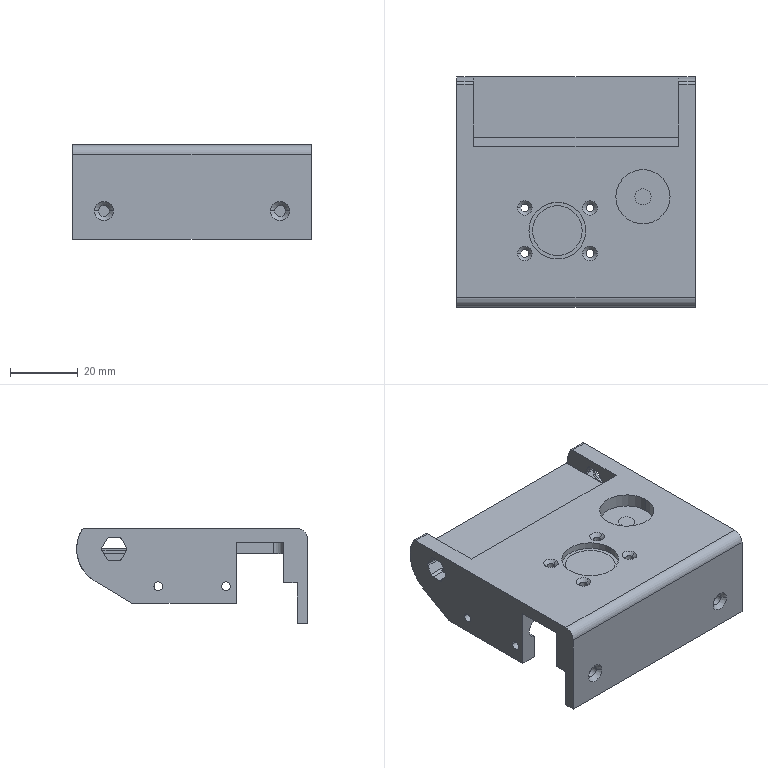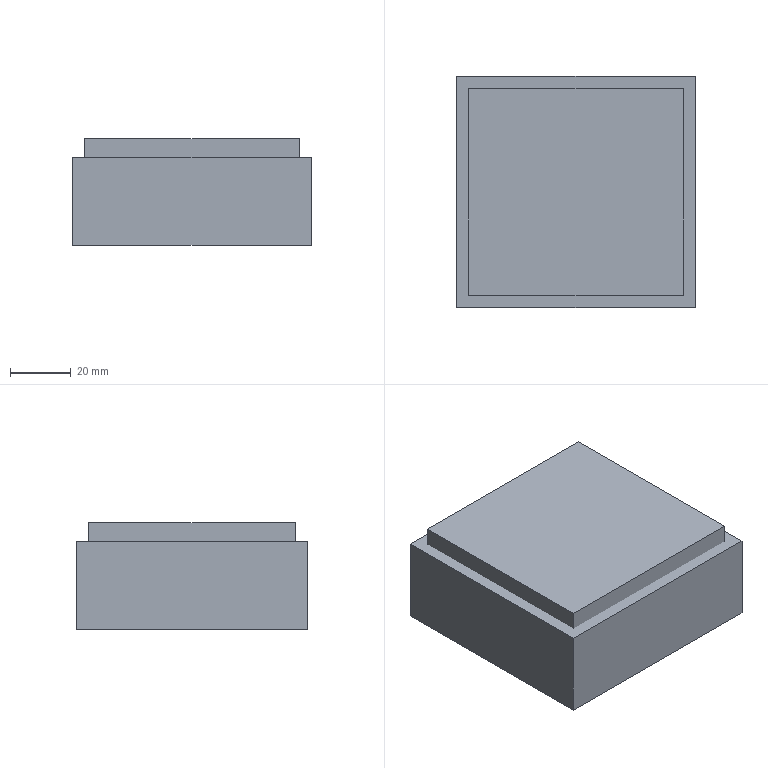CAM job | NX | 3+2 milling, drilling | part box 70.5 x 68.1 x 28 mm | stock box 78.5 x 76.1 x 35 mm
Tools:
number,name,description,diameter,corner_radius,flute_length,length,flutes
1,D63,Milling Tool-5 Parameters,63.0,0.0,50.0,75.0,2
7,D6A45,Milling Tool-5 Parameters,6.0,0.0,3.0,3.0,2
13,3.2ZT,Drilling Tool,3.2,0.0,35.0,50.0,2
12,2.3ZT,Drilling Tool,2.3,0.0,35.0,50.0,2
14,4.8ZT,Drilling Tool,4.8,0.0,35.0,50.0,2
10,D10,Milling Tool-5 Parameters,10.0,0.0,50.0,75.0,2
11,D10JING,Milling Tool-5 Parameters,10.0,0.0,50.0,75.0,2
9,D2R0.5,Milling Tool-5 Parameters,2.0,0.5,50.0,75.0,2
4,D4,Milling Tool-5 Parameters,4.0,0.0,50.0,75.0,2
6,D6,Milling Tool-5 Parameters,6.0,0.0,50.0,75.0,2
2,D2,Milling Tool-5 Parameters,2.0,0.0,50.0,75.0,2
5,D6R0.5,Milling Tool-5 Parameters,6.0,0.5,50.0,75.0,2
16,6.0ZT,Drilling Tool,6.0,0.0,35.0,50.0,2
12,2.6ZT,Drilling Tool,2.6,0.0,35.0,50.0,2
17,2.5ZT,Drilling Tool,2.5,0.0,35.0,50.0,2
Operations:
program,operation,operation_type,tool,method,geometry_group,spindle_rpm,surface_speed,feed_per_tooth,feed_cut,feed_plunge,cut_length_mm,path_length_mm,cut_time_min,machine_time_min
1-75-75-25毛胚,FLOOR_WALL,VolumeBased25DMillingOperation,D63,METHOD,A,6500.0,1286.0,0.0962,1250.0,100.0,482.597,536.597,0.3861,0.3915
1-75-75-25毛胚,DRILLING,Operation,D6A45,METHOD,A,3500.0,43.0,0.0357,250.0,0.0,30.9,223.35,0.1236,0.1428
1-75-75-25毛胚,DRILLING_COPY_COPY,Operation,2.3ZT,METHOD,A,2500.0,19.0,0.024,120.0,0.0,36.764,189.628,0.3064,0.3217
1-75-75-25毛胚,DRILLING_COPY_COPY_COPY,Operation,4.8ZT,METHOD,A,2500.0,19.0,0.024,120.0,0.0,13.442,86.884,0.112,0.1194
1-75-75-25毛胚,ADAPTIVE_MILLING,CavityMilling,D10,METHOD,A,9500.0,298.0,0.1579,3000.0,1000.0,5837.721,7450.176,1.978,2.139
1-75-75-25毛胚,HOLE_MILLING,CylinderMilling,D10,METHOD,A,9500.0,298.0,0.1053,2000.0,100.0,225.87,378.029,0.1129,0.1282
1-75-75-25毛胚,HOLE_MILLING_COPY,CylinderMilling,D10,METHOD,A,9500.0,298.0,0.1053,2000.0,100.0,65.455,130.955,0.0327,0.0393
1-75-75-25毛胚,ZLEVEL_PROFILE_1,ZLevelMilling,D10JING,METHOD,A,9500.0,298.0,0.0526,1000.0,100.0,635.228,748.794,0.6352,0.6466
1-75-75-25毛胚,ZLEVEL_PROFILE_1_COPY,ZLevelMilling,D10JING,METHOD,A,9500.0,298.0,0.0526,1000.0,100.0,30.207,95.207,0.0302,0.0367
1-75-75-25毛胚,ZLEVEL_PROFILE_1_COPY_COPY,ZLevelMilling,D10JING,METHOD,A,9500.0,298.0,0.0526,1000.0,100.0,32.414,93.414,0.0324,0.0385
1-75-75-25毛胚,ZLEVEL_PROFILE_1_COPY_COPY_COPY,ZLevelMilling,D10JING,METHOD,A,9500.0,298.0,0.0526,1000.0,100.0,25.226,87.226,0.0252,0.0314
1-75-75-25毛胚,FLOOR_WALL_1,VolumeBased25DMillingOperation,D10JING,METHOD,A,9500.0,298.0,0.0658,1250.0,100.0,323.3,477.906,0.2586,0.2741
1-75-75-25毛胚,CAVITY_MILL_COPY_COPY,CavityMilling,D4,METHOD,A,9500.0,119.0,0.0737,1400.0,1000.0,345.486,803.476,0.2655,0.3113
1-75-75-25毛胚,CAVITY_MILL_COPY_COPY_COPY,CavityMilling,D2,METHOD,A,9500.0,59.0,0.0526,1000.0,1000.0,429.881,1061.337,0.4299,0.493
1-75-75-25毛胚,ZLEVEL_PROFILE_COPY_COPY_1_1_COPY_1,ZLevelMilling,D2R0.5,METHOD,A,9500.0,59.0,0.1053,2000.0,1000.0,4164.504,4229.096,2.083,2.09
1-75-75-25毛胚,ZLEVEL_PROFILE_COPY_COPY_1_COPY_1,ZLevelMilling,D6R0.5,METHOD,A,9500.0,179.0,0.1579,3000.0,1000.0,4405.43,4466.937,1.47,1.476
1-75-75-25毛胚,ZLEVEL_PROFILE_COPY_COPY_1_COPY_1_COPY,ZLevelMilling,D6R0.5,METHOD,A,9500.0,179.0,0.1579,3000.0,1000.0,1807.575,1989.442,0.6058,0.624
1-75-75-25毛胚,ZLEVEL_PROFILE_1_COPY_1_COPY_COPY_COPY_1,ZLevelMilling,D6A45,METHOD,A,9500.0,179.0,0.0526,1000.0,100.0,274.576,779.626,0.2746,0.3251
1-75-75-25毛胚,ZLEVEL_PROFILE_1_COPY_1_COPY_COPY_COPY_1_COPY,ZLevelMilling,D6A45,METHOD,A,9500.0,179.0,0.0526,1000.0,100.0,14.339,82.339,0.0143,0.0211
2,DRILLING_COPY,Operation,D6A45,METHOD,B,3500.0,43.0,0.0357,250.0,0.0,10.3,142.676,0.0412,0.0544
2,DRILLING_COPY_COPY_COPY_COPY,Operation,6.0ZT,METHOD,B,2500.0,19.0,0.024,120.0,0.0,82.705,287.486,0.6892,0.7097
3,DRILLING_1,Operation,D6A45,METHOD,C,3500.0,43.0,0.0357,250.0,0.0,11.6,138.286,0.0464,0.0591
3,DRILLING_COPY_COPY_1,Operation,3.2ZT,METHOD,C,2500.0,19.0,0.024,120.0,0.0,16.923,148.932,0.141,0.1542
4,DRILLING_COPY_1,Operation,D6A45,METHOD,D,3500.0,43.0,0.0357,250.0,0.0,8.8,100.824,0.0352,0.0444
4,DRILLING_COPY_COPY_COPY_1,Operation,2.6ZT,METHOD,D,2500.0,19.0,0.024,120.0,0.0,20.562,124.348,0.1714,0.1817
4,ZLEVEL_PROFILE_COPY,ZLevelMilling,D2,METHOD,D,9500.0,59.0,0.0526,1000.0,1000.0,595.828,658.828,0.5958,0.6021
4,ZLEVEL_PROFILE_1_COPY_1_COPY_COPY_COPY_1_COPY_COPY,ZLevelMilling,D6A45,METHOD,D,9500.0,179.0,0.0526,1000.0,100.0,33.118,264.656,0.0331,0.0563
5,DRILLING_COPY_2,Operation,D6A45,METHOD,E,3500.0,43.0,0.0357,250.0,0.0,12.0,156.733,0.048,0.0625
5,DRILLING_COPY_COPY_COPY_2,Operation,2.5ZT,METHOD,E,2500.0,19.0,0.024,120.0,0.0,11.5,83.0,0.0958,0.103
5,DRILLING_COPY_COPY_COPY_1_COPY,Operation,2.6ZT,METHOD,E,2500.0,19.0,0.024,120.0,0.0,10.281,80.562,0.0857,0.0927
5,ZLEVEL_PROFILE_COPY_COPY,ZLevelMilling,D4,METHOD,E,9500.0,119.0,0.0684,1300.0,1000.0,252.739,316.306,0.2058,0.2122
5,ZLEVEL_PROFILE_COPY_COPY_1,ZLevelMilling,D2R0.5,METHOD,E,9500.0,59.0,0.0789,1500.0,1000.0,1038.406,1101.906,0.6993,0.7056
5,ZLEVEL_PROFILE_1_COPY_1_COPY_COPY_COPY_1_COPY_COPY_COPY,ZLevelMilling,D6A45,METHOD,E,9500.0,179.0,0.0526,1000.0,100.0,36.649,315.718,0.0366,0.0646
5,刀补4,ZLevelMilling,D4,METHOD,E,9500.0,119.0,0.0526,1000.0,100.0,17.875,76.34,0.0179,0.0237
6,FLOOR_WALL_COPY,VolumeBased25DMillingOperation,D63,METHOD,F,6500.0,1286.0,0.0962,1250.0,100.0,2236.479,2844.263,1.789,1.85
6,FLOOR_WALL_2,VolumeBased25DMillingOperation,D10,METHOD,F,9500.0,298.0,0.1579,3000.0,1000.0,5409.407,5475.107,1.807,1.814
6,ADAPTIVE_MILLING_COPY,CavityMilling,D10,METHOD,F,9500.0,298.0,0.1579,3000.0,1000.0,10554.564,17811.647,3.646,4.372
6,HOLE_MILLING_COPY_COPY,CylinderMilling,D10,METHOD,F,9500.0,298.0,0.1053,2000.0,100.0,82.977,191.977,0.0415,0.0524
6,ZLEVEL_PROFILE_2,ZLevelMilling,D10,METHOD,MCS_MILL_-F,9500.0,298.0,0.1053,2000.0,100.0,178.605,282.938,0.0893,0.0997
6,FLOOR_WALL_1_COPY,VolumeBased25DMillingOperation,D10JING,METHOD,F,9500.0,298.0,0.0658,1250.0,100.0,1481.938,3039.233,1.186,1.341
6,ZLEVEL_PROFILE,ZLevelMilling,D6,METHOD,F,9500.0,179.0,0.0842,1600.0,100.0,134.03,562.062,0.0838,0.1266
6,ZLEVEL_PROFILE_COPY_1,ZLevelMilling,D6,METHOD,MCS_MILL_-F,9500.0,179.0,0.0842,1600.0,100.0,63.904,345.959,0.0399,0.0681
6,ZLEVEL_PROFILE_COPY_COPY_1_COPY_1_COPY_1,ZLevelMilling,D6R0.5,METHOD,F,9500.0,179.0,0.1579,3000.0,1000.0,5765.42,6006.058,1.925,1.949
6,ZLEVEL_PROFILE_1_COPY_1_COPY_COPY_COPY_1_COPY_COPY_COPY_COPY,ZLevelMilling,D6A45,METHOD,F,9500.0,179.0,0.0526,1000.0,100.0,158.1,218.1,0.1581,0.1641
6,ZLEVEL_PROFILE_1_COPY_1_COPY_COPY_COPY_1_COPY_COPY_COPY_COPY_COPY,ZLevelMilling,D6A45,METHOD,F,9500.0,179.0,0.0526,1000.0,100.0,80.276,164.276,0.0803,0.0887
6,ZLEVEL_PROFILE_1_COPY_1_COPY_COPY_COPY_1_COPY_COPY_COPY_COPY_COPY_COPY,ZLevelMilling,D6A45,METHOD,F,9500.0,179.0,0.0526,1000.0,100.0,98.258,317.38,0.0983,0.1202
6,ZLEVEL_PROFILE_1_COPY_1_COPY_COPY_COPY_1_COPY_COPY_COPY_COPY_COPY_COPY_COPY,ZLevelMilling,D6A45,METHOD,F,9500.0,179.0,0.0526,1000.0,100.0,170.877,532.784,0.1709,0.2071
6,ZLEVEL_PROFILE_1_COPY_1_COPY_COPY_COPY_1_COPY_COPY_COPY_COPY_COPY_COPY_COPY_COPY,ZLevelMilling,D6A45,METHOD,F,9500.0,179.0,0.0526,1000.0,100.0,82.977,812.441,0.083,0.1559
7,FLOOR_WALL_1_COPY_1,VolumeBased25DMillingOperation,D10JING,METHOD,G,9500.0,298.0,0.0658,1250.0,100.0,216.109,512.374,0.1729,0.2025